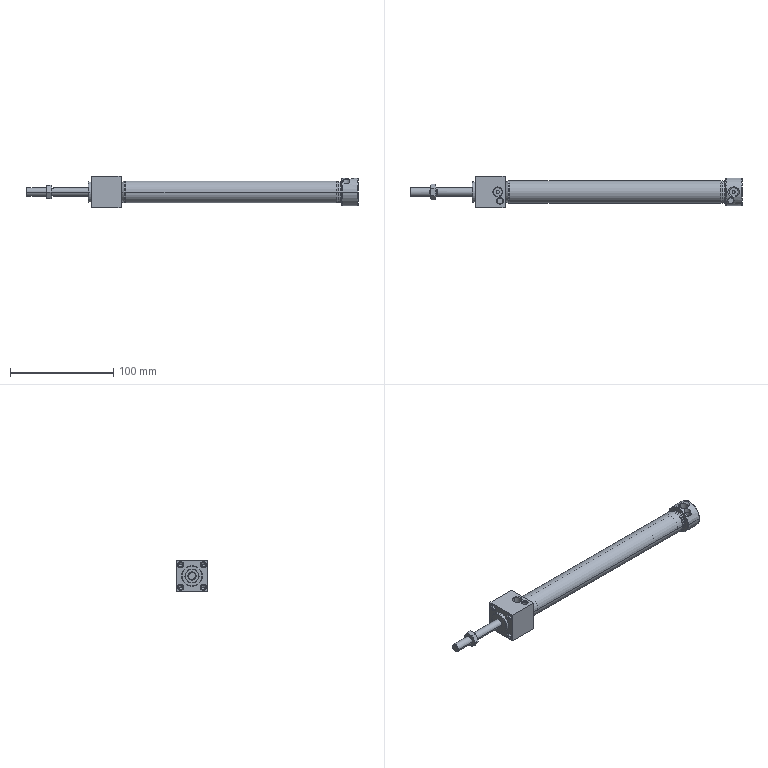Part | SolidWorks | 3 solids | 142 faces | box 322.308 x 30.5 x 30.5 mm | volume 65420 mm3 | cylinder 47 | cone 44 | plane 37 | torus 14 | commonest cylinder face diameters 4.134 x8 21.4 x6 3 x4 5.5 x4 8 x4 8.566 x4